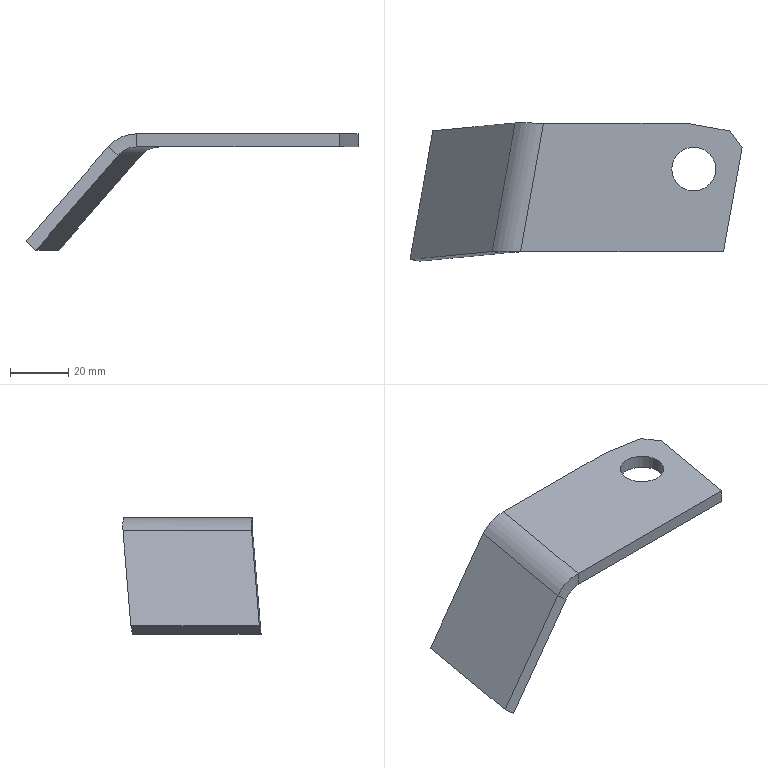Part | SolidWorks | features FlatPattern 1, SM3dBend 1, SMBaseFlange 1, SheetMetal 1 | 1 solid | 18 faces | box 113.633 x 47.299 x 39.859 mm | volume 23066 mm3 | plane 12 | cylinder 4 | spline 2 | commonest cylinder face diameters 15 x2 16 x1 25 x1
STEP:
#1=CARTESIAN_POINT('',(103.623,28.367,-4.5));
#2=VERTEX_POINT('',#1);
#3=CARTESIAN_POINT('',(118.623,28.367,-4.5));
#4=VERTEX_POINT('',#3);
#5=CARTESIAN_POINT('',(111.123,28.367,-4.5));
#6=DIRECTION('',(0.,0.,1.));
#7=DIRECTION('',(1.,0.,0.));
#8=AXIS2_PLACEMENT_3D('',#5,#6,#7);
#9=CIRCLE('',#8,7.5);
#10=EDGE_CURVE('',#2,#4,#9,.T.);
#11=ORIENTED_EDGE('',*,*,#10,.F.);
#12=CARTESIAN_POINT('',(103.623,28.367,0.));
#13=VERTEX_POINT('',#12);
#14=CARTESIAN_POINT('',(103.623,28.367,-4.5));
#15=DIRECTION('',(0.,0.,1.));
#16=VECTOR('',#15,1000.);
#17=LINE('',#14,#16);
#18=EDGE_CURVE('',#2,#13,#17,.T.);
#19=ORIENTED_EDGE('',*,*,#18,.T.);
#20=CARTESIAN_POINT('',(118.623,28.367,0.));
#21=VERTEX_POINT('',#20);
#22=CARTESIAN_POINT('',(111.123,28.367,0.));
#23=DIRECTION('',(0.,0.,1.));
#24=DIRECTION('',(1.,0.,0.));
#25=AXIS2_PLACEMENT_3D('',#22,#23,#24);
#26=CIRCLE('',#25,7.5);
#27=EDGE_CURVE('',#13,#21,#26,.T.);
#28=ORIENTED_EDGE('',*,*,#27,.T.);
#29=CARTESIAN_POINT('',(118.623,28.367,-4.5));
#30=DIRECTION('',(0.,0.,1.));
#31=VECTOR('',#30,1000.);
#32=LINE('',#29,#31);
#33=EDGE_CURVE('',#4,#21,#32,.T.);
#34=ORIENTED_EDGE('',*,*,#33,.F.);
#35=EDGE_LOOP('',(#11,#19,#28,#34));
#36=FACE_OUTER_BOUND('',#35,.T.);
#37=CARTESIAN_POINT('',(111.123,28.367,-4.5));
#38=DIRECTION('',(0.,0.,1.));
#39=DIRECTION('',(1.,0.,0.));
#40=AXIS2_PLACEMENT_3D('',#37,#38,#39);
#41=CYLINDRICAL_SURFACE('',#40,7.5);
#42=ADVANCED_FACE('',(#36),#41,.F.);
#43=CARTESIAN_POINT('',(53.399,43.554,-7.358));
#44=VERTEX_POINT('',#43);
#45=CARTESIAN_POINT('',(25.222,40.893,-39.859));
#46=VERTEX_POINT('',#45);
#47=CARTESIAN_POINT('',(91.322,47.135,36.385));
#48=DIRECTION('',(-0.6538,-0.06175,-0.7541));
#49=VECTOR('',#48,1000.);
#50=LINE('',#47,#49);
#51=EDGE_CURVE('',#44,#46,#50,.T.);
#52=ORIENTED_EDGE('',*,*,#51,.F.);
#53=CARTESIAN_POINT('',(45.551,-0.4463,-7.358));
#54=VERTEX_POINT('',#53);
#55=CARTESIAN_POINT('',(44.224,-7.888,-7.358));
#56=DIRECTION('',(-0.1756,-0.9845,0.));
#57=VECTOR('',#56,1000.);
#58=LINE('',#55,#57);
#59=EDGE_CURVE('',#44,#54,#58,.T.);
#60=ORIENTED_EDGE('',*,*,#59,.T.);
#61=CARTESIAN_POINT('',(17.406,-3.104,-39.823));
#62=VERTEX_POINT('',#61);
#63=CARTESIAN_POINT('',(17.406,-3.104,-39.823));
#64=DIRECTION('',(0.6538,0.06175,0.7541));
#65=VECTOR('',#64,1000.);
#66=LINE('',#63,#65);
#67=EDGE_CURVE('',#62,#54,#66,.T.);
#68=ORIENTED_EDGE('',*,*,#67,.F.);
#69=CARTESIAN_POINT('',(25.222,40.893,-39.859));
#70=DIRECTION('',(-0.1749,-0.9846,0.0008057));
#71=VECTOR('',#70,1000.);
#72=LINE('',#69,#71);
#73=EDGE_CURVE('',#46,#62,#72,.T.);
#74=ORIENTED_EDGE('',*,*,#73,.F.);
#75=EDGE_LOOP('',(#52,#60,#68,#74));
#76=FACE_OUTER_BOUND('',#75,.T.);
#77=CARTESIAN_POINT('',(17.406,-3.104,-39.823));
#78=DIRECTION('',(-0.7541,0.1345,0.6428));
#79=DIRECTION('',(0.6538,0.06175,0.7541));
#80=AXIS2_PLACEMENT_3D('',#77,#78,#79);
#81=PLANE('',#80);
#82=ADVANCED_FACE('',(#76),#81,.F.);
#83=CARTESIAN_POINT('',(21.829,41.498,-36.967));
#84=VERTEX_POINT('',#83);
#85=CARTESIAN_POINT('',(14.012,-2.499,-36.931));
#86=VERTEX_POINT('',#85);
#87=CARTESIAN_POINT('',(21.829,41.498,-36.967));
#88=DIRECTION('',(-0.1749,-0.9846,0.0008057));
#89=VECTOR('',#88,1000.);
#90=LINE('',#87,#89);
#91=EDGE_CURVE('',#84,#86,#90,.T.);
#92=ORIENTED_EDGE('',*,*,#91,.F.);
#93=CARTESIAN_POINT('',(25.222,40.893,-39.859));
#94=DIRECTION('',(-0.7541,0.1345,0.6428));
#95=VECTOR('',#94,1000.);
#96=LINE('',#93,#95);
#97=EDGE_CURVE('',#46,#84,#96,.T.);
#98=ORIENTED_EDGE('',*,*,#97,.F.);
#99=ORIENTED_EDGE('',*,*,#73,.T.);
#100=CARTESIAN_POINT('',(17.406,-3.104,-39.823));
#101=DIRECTION('',(-0.7541,0.1345,0.6428));
#102=VECTOR('',#101,1000.);
#103=LINE('',#100,#102);
#104=EDGE_CURVE('',#62,#86,#103,.T.);
#105=ORIENTED_EDGE('',*,*,#104,.T.);
#106=EDGE_LOOP('',(#92,#98,#99,#105));
#107=FACE_OUTER_BOUND('',#106,.T.);
#108=CARTESIAN_POINT('',(25.222,40.893,-39.859));
#109=DIRECTION('',(-0.633,0.1118,-0.766));
#110=DIRECTION('',(-0.1749,-0.9846,0.0008057));
#111=AXIS2_PLACEMENT_3D('',#108,#109,#110);
#112=PLANE('',#111);
#113=ADVANCED_FACE('',(#107),#112,.T.);
#114=CARTESIAN_POINT('',(50.006,44.159,-4.465));
#115=VERTEX_POINT('',#114);
#116=CARTESIAN_POINT('',(53.399,43.554,-7.358));
#117=CARTESIAN_POINT('',(50.006,44.159,-4.465));
#118=B_SPLINE_CURVE_WITH_KNOTS('',1,(#116,#117),.UNSPECIFIED.,.F.,.F.,(2,2),(0.,1.),.UNSPECIFIED.);
#119=EDGE_CURVE('',#44,#115,#118,.T.);
#120=ORIENTED_EDGE('',*,*,#119,.F.);
#121=ORIENTED_EDGE('',*,*,#51,.T.);
#122=ORIENTED_EDGE('',*,*,#97,.T.);
#123=CARTESIAN_POINT('',(87.928,47.741,39.277));
#124=DIRECTION('',(-0.6538,-0.06175,-0.7541));
#125=VECTOR('',#124,1000.);
#126=LINE('',#123,#125);
#127=EDGE_CURVE('',#115,#84,#126,.T.);
#128=ORIENTED_EDGE('',*,*,#127,.F.);
#129=EDGE_LOOP('',(#120,#121,#122,#128));
#130=FACE_OUTER_BOUND('',#129,.T.);
#131=CARTESIAN_POINT('',(91.322,47.135,36.385));
#132=DIRECTION('',(0.06175,0.989,-0.1345));
#133=DIRECTION('',(-0.6538,-0.06175,-0.7541));
#134=AXIS2_PLACEMENT_3D('',#131,#132,#133);
#135=PLANE('',#134);
#136=ADVANCED_FACE('',(#130),#135,.T.);
#137=CARTESIAN_POINT('',(42.158,0.159,-4.465));
#138=VERTEX_POINT('',#137);
#139=CARTESIAN_POINT('',(42.158,0.159,-4.465));
#140=CARTESIAN_POINT('',(45.551,-0.4463,-7.358));
#141=B_SPLINE_CURVE_WITH_KNOTS('',1,(#139,#140),.UNSPECIFIED.,.F.,.F.,(2,2),(0.,1.),.UNSPECIFIED.);
#142=EDGE_CURVE('',#138,#54,#141,.T.);
#143=ORIENTED_EDGE('',*,*,#142,.F.);
#144=CARTESIAN_POINT('',(14.012,-2.499,-36.931));
#145=DIRECTION('',(0.6538,0.06175,0.7541));
#146=VECTOR('',#145,1000.);
#147=LINE('',#144,#146);
#148=EDGE_CURVE('',#86,#138,#147,.T.);
#149=ORIENTED_EDGE('',*,*,#148,.F.);
#150=ORIENTED_EDGE('',*,*,#104,.F.);
#151=ORIENTED_EDGE('',*,*,#67,.T.);
#152=EDGE_LOOP('',(#143,#149,#150,#151));
#153=FACE_OUTER_BOUND('',#152,.T.);
#154=CARTESIAN_POINT('',(17.406,-3.104,-39.823));
#155=DIRECTION('',(-0.06175,-0.989,0.1345));
#156=DIRECTION('',(0.7541,-0.1345,-0.6428));
#157=AXIS2_PLACEMENT_3D('',#154,#155,#156);
#158=PLANE('',#157);
#159=ADVANCED_FACE('',(#153),#158,.T.);
#160=CARTESIAN_POINT('',(40.831,-7.282,-4.465));
#161=DIRECTION('',(-0.1756,-0.9845,0.));
#162=VECTOR('',#161,1000.);
#163=LINE('',#160,#162);
#164=EDGE_CURVE('',#115,#138,#163,.T.);
#165=ORIENTED_EDGE('',*,*,#164,.F.);
#166=ORIENTED_EDGE('',*,*,#127,.T.);
#167=ORIENTED_EDGE('',*,*,#91,.T.);
#168=ORIENTED_EDGE('',*,*,#148,.T.);
#169=EDGE_LOOP('',(#165,#166,#167,#168));
#170=FACE_OUTER_BOUND('',#169,.T.);
#171=CARTESIAN_POINT('',(14.012,-2.499,-36.931));
#172=DIRECTION('',(-0.7541,0.1345,0.6428));
#173=DIRECTION('',(0.6538,0.06175,0.7541));
#174=AXIS2_PLACEMENT_3D('',#171,#172,#173);
#175=PLANE('',#174);
#176=ADVANCED_FACE('',(#170),#175,.T.);
#177=ORIENTED_EDGE('',*,*,#18,.F.);
#178=CARTESIAN_POINT('',(111.123,28.367,-4.5));
#179=DIRECTION('',(0.,0.,1.));
#180=DIRECTION('',(1.,0.,0.));
#181=AXIS2_PLACEMENT_3D('',#178,#179,#180);
#182=CIRCLE('',#181,7.5);
#183=EDGE_CURVE('',#4,#2,#182,.T.);
#184=ORIENTED_EDGE('',*,*,#183,.F.);
#185=ORIENTED_EDGE('',*,*,#33,.T.);
#186=CARTESIAN_POINT('',(111.123,28.367,0.));
#187=DIRECTION('',(0.,0.,1.));
#188=DIRECTION('',(1.,0.,0.));
#189=AXIS2_PLACEMENT_3D('',#186,#187,#188);
#190=CIRCLE('',#189,7.5);
#191=EDGE_CURVE('',#21,#13,#190,.T.);
#192=ORIENTED_EDGE('',*,*,#191,.T.);
#193=EDGE_LOOP('',(#177,#184,#185,#192));
#194=FACE_OUTER_BOUND('',#193,.T.);
#195=CARTESIAN_POINT('',(111.123,28.367,-4.5));
#196=DIRECTION('',(0.,0.,1.));
#197=DIRECTION('',(1.,0.,0.));
#198=AXIS2_PLACEMENT_3D('',#195,#196,#197);
#199=CYLINDRICAL_SURFACE('',#198,7.5);
#200=ADVANCED_FACE('',(#194),#199,.F.);
#201=CARTESIAN_POINT('',(121.3,0.,0.));
#202=VERTEX_POINT('',#201);
#203=CARTESIAN_POINT('',(127.646,35.578,0.));
#204=VERTEX_POINT('',#203);
#205=CARTESIAN_POINT('',(121.3,0.,0.));
#206=DIRECTION('',(0.1756,0.9845,0.));
#207=VECTOR('',#206,1000.);
#208=LINE('',#205,#207);
#209=EDGE_CURVE('',#202,#204,#208,.T.);
#210=ORIENTED_EDGE('',*,*,#209,.F.);
#211=CARTESIAN_POINT('',(121.3,0.,-4.5));
#212=VERTEX_POINT('',#211);
#213=CARTESIAN_POINT('',(121.3,0.,-4.5));
#214=DIRECTION('',(0.,0.,1.));
#215=VECTOR('',#214,1000.);
#216=LINE('',#213,#215);
#217=EDGE_CURVE('',#212,#202,#216,.T.);
#218=ORIENTED_EDGE('',*,*,#217,.F.);
#219=CARTESIAN_POINT('',(127.646,35.578,-4.5));
#220=VERTEX_POINT('',#219);
#221=CARTESIAN_POINT('',(121.3,0.,-4.5));
#222=DIRECTION('',(0.1756,0.9845,0.));
#223=VECTOR('',#222,1000.);
#224=LINE('',#221,#223);
#225=EDGE_CURVE('',#212,#220,#224,.T.);
#226=ORIENTED_EDGE('',*,*,#225,.T.);
#227=CARTESIAN_POINT('',(127.646,35.578,-4.5));
#228=DIRECTION('',(0.,0.,1.));
#229=VECTOR('',#228,1000.);
#230=LINE('',#227,#229);
#231=EDGE_CURVE('',#220,#204,#230,.T.);
#232=ORIENTED_EDGE('',*,*,#231,.T.);
#233=EDGE_LOOP('',(#210,#218,#226,#232));
#234=FACE_OUTER_BOUND('',#233,.T.);
#235=CARTESIAN_POINT('',(121.3,0.,-4.5));
#236=DIRECTION('',(0.9845,-0.1756,0.));
#237=DIRECTION('',(0.1756,0.9845,0.));
#238=AXIS2_PLACEMENT_3D('',#235,#236,#237);
#239=PLANE('',#238);
#240=ADVANCED_FACE('',(#234),#239,.T.);
#241=CARTESIAN_POINT('',(123.601,41.378,0.));
#242=VERTEX_POINT('',#241);
#243=CARTESIAN_POINT('',(123.601,41.378,0.));
#244=DIRECTION('',(-0.572,0.8203,0.));
#245=VECTOR('',#244,1000.);
#246=LINE('',#243,#245);
#247=EDGE_CURVE('',#204,#242,#246,.T.);
#248=ORIENTED_EDGE('',*,*,#247,.F.);
#249=ORIENTED_EDGE('',*,*,#231,.F.);
#250=CARTESIAN_POINT('',(123.601,41.378,-4.5));
#251=VERTEX_POINT('',#250);
#252=CARTESIAN_POINT('',(123.601,41.378,-4.5));
#253=DIRECTION('',(-0.572,0.8203,0.));
#254=VECTOR('',#253,1000.);
#255=LINE('',#252,#254);
#256=EDGE_CURVE('',#220,#251,#255,.T.);
#257=ORIENTED_EDGE('',*,*,#256,.T.);
#258=CARTESIAN_POINT('',(123.601,41.378,-4.5));
#259=DIRECTION('',(0.,0.,1.));
#260=VECTOR('',#259,1000.);
#261=LINE('',#258,#260);
#262=EDGE_CURVE('',#251,#242,#261,.T.);
#263=ORIENTED_EDGE('',*,*,#262,.T.);
#264=EDGE_LOOP('',(#248,#249,#257,#263));
#265=FACE_OUTER_BOUND('',#264,.T.);
#266=CARTESIAN_POINT('',(123.601,41.378,-4.5));
#267=DIRECTION('',(0.8203,0.572,0.));
#268=DIRECTION('',(-0.572,0.8203,0.));
#269=AXIS2_PLACEMENT_3D('',#266,#267,#268);
#270=PLANE('',#269);
#271=ADVANCED_FACE('',(#265),#270,.T.);
#272=CARTESIAN_POINT('',(108.9,44.,0.));
#273=VERTEX_POINT('',#272);
#274=CARTESIAN_POINT('',(108.9,44.,0.));
#275=DIRECTION('',(-0.9845,0.1756,0.));
#276=VECTOR('',#275,1000.);
#277=LINE('',#274,#276);
#278=EDGE_CURVE('',#242,#273,#277,.T.);
#279=ORIENTED_EDGE('',*,*,#278,.F.);
#280=ORIENTED_EDGE('',*,*,#262,.F.);
#281=CARTESIAN_POINT('',(108.9,44.,-4.5));
#282=VERTEX_POINT('',#281);
#283=CARTESIAN_POINT('',(108.9,44.,-4.5));
#284=DIRECTION('',(-0.9845,0.1756,0.));
#285=VECTOR('',#284,1000.);
#286=LINE('',#283,#285);
#287=EDGE_CURVE('',#251,#282,#286,.T.);
#288=ORIENTED_EDGE('',*,*,#287,.T.);
#289=CARTESIAN_POINT('',(108.9,44.,-4.5));
#290=DIRECTION('',(0.,0.,1.));
#291=VECTOR('',#290,1000.);
#292=LINE('',#289,#291);
#293=EDGE_CURVE('',#282,#273,#292,.T.);
#294=ORIENTED_EDGE('',*,*,#293,.T.);
#295=EDGE_LOOP('',(#279,#280,#288,#294));
#296=FACE_OUTER_BOUND('',#295,.T.);
#297=CARTESIAN_POINT('',(108.9,44.,-4.5));
#298=DIRECTION('',(0.1756,0.9845,0.));
#299=DIRECTION('',(-0.9845,0.1756,0.));
#300=AXIS2_PLACEMENT_3D('',#297,#298,#299);
#301=PLANE('',#300);
#302=ADVANCED_FACE('',(#296),#301,.T.);
#303=CARTESIAN_POINT('',(59.704,44.,-4.5));
#304=VERTEX_POINT('',#303);
#305=CARTESIAN_POINT('',(51.856,0.,-4.5));
#306=VERTEX_POINT('',#305);
#307=CARTESIAN_POINT('',(50.257,-8.964,-4.5));
#308=DIRECTION('',(-0.1756,-0.9845,0.));
#309=VECTOR('',#308,1000.);
#310=LINE('',#307,#309);
#311=EDGE_CURVE('',#304,#306,#310,.T.);
#312=ORIENTED_EDGE('',*,*,#311,.F.);
#313=CARTESIAN_POINT('',(108.9,44.,-4.5));
#314=DIRECTION('',(-1.,0.,0.));
#315=VECTOR('',#314,1000.);
#316=LINE('',#313,#315);
#317=EDGE_CURVE('',#282,#304,#316,.T.);
#318=ORIENTED_EDGE('',*,*,#317,.F.);
#319=ORIENTED_EDGE('',*,*,#287,.F.);
#320=ORIENTED_EDGE('',*,*,#256,.F.);
#321=ORIENTED_EDGE('',*,*,#225,.F.);
#322=CARTESIAN_POINT('',(0.,0.,-4.5));
#323=DIRECTION('',(1.,0.,0.));
#324=VECTOR('',#323,1000.);
#325=LINE('',#322,#324);
#326=EDGE_CURVE('',#306,#212,#325,.T.);
#327=ORIENTED_EDGE('',*,*,#326,.F.);
#328=EDGE_LOOP('',(#312,#318,#319,#320,#321,#327));
#329=FACE_OUTER_BOUND('',#328,.T.);
#330=ORIENTED_EDGE('',*,*,#183,.T.);
#331=ORIENTED_EDGE('',*,*,#10,.T.);
#332=EDGE_LOOP('',(#330,#331));
#333=FACE_BOUND('',#332,.T.);
#334=CARTESIAN_POINT('',(0.,0.,-4.5));
#335=DIRECTION('',(0.,0.,1.));
#336=DIRECTION('',(1.,0.,0.));
#337=AXIS2_PLACEMENT_3D('',#334,#335,#336);
#338=PLANE('',#337);
#339=ADVANCED_FACE('',(#329,#333),#338,.F.);
#340=ORIENTED_EDGE('',*,*,#317,.T.);
#341=CARTESIAN_POINT('',(59.704,44.,0.));
#342=VERTEX_POINT('',#341);
#343=CARTESIAN_POINT('',(59.704,44.,-4.5));
#344=CARTESIAN_POINT('',(59.704,44.,-3.));
#345=CARTESIAN_POINT('',(59.704,44.,-1.5));
#346=CARTESIAN_POINT('',(59.704,44.,0.));
#347=B_SPLINE_CURVE_WITH_KNOTS('',3,(#343,#344,#345,#346),.UNSPECIFIED.,.F.,.F.,(4,4),(0.,1.),.UNSPECIFIED.);
#348=EDGE_CURVE('',#304,#342,#347,.T.);
#349=ORIENTED_EDGE('',*,*,#348,.T.);
#350=CARTESIAN_POINT('',(108.9,44.,0.));
#351=DIRECTION('',(-1.,0.,0.));
#352=VECTOR('',#351,1000.);
#353=LINE('',#350,#352);
#354=EDGE_CURVE('',#273,#342,#353,.T.);
#355=ORIENTED_EDGE('',*,*,#354,.F.);
#356=ORIENTED_EDGE('',*,*,#293,.F.);
#357=EDGE_LOOP('',(#340,#349,#355,#356));
#358=FACE_OUTER_BOUND('',#357,.T.);
#359=CARTESIAN_POINT('',(108.9,44.,-4.5));
#360=DIRECTION('',(0.,1.,0.));
#361=DIRECTION('',(-1.,0.,0.));
#362=AXIS2_PLACEMENT_3D('',#359,#360,#361);
#363=PLANE('',#362);
#364=ADVANCED_FACE('',(#358),#363,.T.);
#365=ORIENTED_EDGE('',*,*,#191,.F.);
#366=ORIENTED_EDGE('',*,*,#27,.F.);
#367=EDGE_LOOP('',(#365,#366));
#368=FACE_BOUND('',#367,.T.);
#369=ORIENTED_EDGE('',*,*,#354,.T.);
#370=CARTESIAN_POINT('',(51.856,0.,0.));
#371=VERTEX_POINT('',#370);
#372=CARTESIAN_POINT('',(50.257,-8.964,0.));
#373=DIRECTION('',(-0.1756,-0.9845,0.));
#374=VECTOR('',#373,1000.);
#375=LINE('',#372,#374);
#376=EDGE_CURVE('',#342,#371,#375,.T.);
#377=ORIENTED_EDGE('',*,*,#376,.T.);
#378=CARTESIAN_POINT('',(0.,0.,0.));
#379=DIRECTION('',(1.,0.,0.));
#380=VECTOR('',#379,1000.);
#381=LINE('',#378,#380);
#382=EDGE_CURVE('',#371,#202,#381,.T.);
#383=ORIENTED_EDGE('',*,*,#382,.T.);
#384=ORIENTED_EDGE('',*,*,#209,.T.);
#385=ORIENTED_EDGE('',*,*,#247,.T.);
#386=ORIENTED_EDGE('',*,*,#278,.T.);
#387=EDGE_LOOP('',(#369,#377,#383,#384,#385,#386));
#388=FACE_OUTER_BOUND('',#387,.T.);
#389=CARTESIAN_POINT('',(0.,0.,0.));
#390=DIRECTION('',(0.,0.,1.));
#391=DIRECTION('',(1.,0.,0.));
#392=AXIS2_PLACEMENT_3D('',#389,#390,#391);
#393=PLANE('',#392);
#394=ADVANCED_FACE('',(#368,#388),#393,.T.);
#395=ORIENTED_EDGE('',*,*,#382,.F.);
#396=CARTESIAN_POINT('',(51.856,0.,0.));
#397=CARTESIAN_POINT('',(51.856,0.,-1.5));
#398=CARTESIAN_POINT('',(51.856,0.,-3.));
#399=CARTESIAN_POINT('',(51.856,0.,-4.5));
#400=B_SPLINE_CURVE_WITH_KNOTS('',3,(#396,#397,#398,#399),.UNSPECIFIED.,.F.,.F.,(4,4),(0.,1.),.UNSPECIFIED.);
#401=EDGE_CURVE('',#371,#306,#400,.T.);
#402=ORIENTED_EDGE('',*,*,#401,.T.);
#403=ORIENTED_EDGE('',*,*,#326,.T.);
#404=ORIENTED_EDGE('',*,*,#217,.T.);
#405=EDGE_LOOP('',(#395,#402,#403,#404));
#406=FACE_OUTER_BOUND('',#405,.T.);
#407=CARTESIAN_POINT('',(0.,0.,-4.5));
#408=DIRECTION('',(0.,-1.,0.));
#409=DIRECTION('',(0.,0.,-1.));
#410=AXIS2_PLACEMENT_3D('',#407,#408,#409);
#411=PLANE('',#410);
#412=ADVANCED_FACE('',(#406),#411,.T.);
#413=ORIENTED_EDGE('',*,*,#119,.T.);
#414=CARTESIAN_POINT('',(50.006,44.159,-4.465));
#415=CARTESIAN_POINT('',(51.202,44.208,-3.072));
#416=CARTESIAN_POINT('',(52.7,44.202,-1.939));
#417=CARTESIAN_POINT('',(56.035,44.131,-0.4028));
#418=CARTESIAN_POINT('',(57.868,44.066,0.));
#419=CARTESIAN_POINT('',(59.704,44.,0.));
#420=B_SPLINE_CURVE_WITH_KNOTS('',3,(#414,#415,#416,#417,#418,#419),.UNSPECIFIED.,.F.,.F.,(4,2,4),(0.,0.5,1.),.UNSPECIFIED.);
#421=EDGE_CURVE('',#115,#342,#420,.T.);
#422=ORIENTED_EDGE('',*,*,#421,.T.);
#423=ORIENTED_EDGE('',*,*,#348,.F.);
#424=CARTESIAN_POINT('',(53.399,43.554,-7.358));
#425=CARTESIAN_POINT('',(54.181,43.676,-6.466));
#426=CARTESIAN_POINT('',(55.156,43.764,-5.741));
#427=CARTESIAN_POINT('',(57.323,43.901,-4.758));
#428=CARTESIAN_POINT('',(58.513,43.951,-4.5));
#429=CARTESIAN_POINT('',(59.704,44.,-4.5));
#430=B_SPLINE_CURVE_WITH_KNOTS('',3,(#424,#425,#426,#427,#428,#429),.UNSPECIFIED.,.F.,.F.,(4,2,4),(0.,0.5,1.),.UNSPECIFIED.);
#431=EDGE_CURVE('',#44,#304,#430,.T.);
#432=ORIENTED_EDGE('',*,*,#431,.F.);
#433=EDGE_LOOP('',(#413,#422,#423,#432));
#434=FACE_OUTER_BOUND('',#433,.T.);
#435=CARTESIAN_POINT('',(50.006,44.159,-4.465));
#436=CARTESIAN_POINT('',(51.202,44.208,-3.072));
#437=CARTESIAN_POINT('',(52.7,44.202,-1.939));
#438=CARTESIAN_POINT('',(56.035,44.131,-0.4028));
#439=CARTESIAN_POINT('',(57.868,44.066,0.));
#440=CARTESIAN_POINT('',(59.704,44.,0.));
#441=CARTESIAN_POINT('',(53.399,43.554,-7.358));
#442=CARTESIAN_POINT('',(54.181,43.676,-6.466));
#443=CARTESIAN_POINT('',(55.156,43.764,-5.741));
#444=CARTESIAN_POINT('',(57.323,43.901,-4.758));
#445=CARTESIAN_POINT('',(58.513,43.951,-4.5));
#446=CARTESIAN_POINT('',(59.704,44.,-4.5));
#447=B_SPLINE_SURFACE_WITH_KNOTS('',1,3,((#435,#436,#437,#438,#439,#440),(#441,#442,#443,#444,#445,#446)),.UNSPECIFIED.,.F.,.F.,.F.,(2,2),(4,2,4),(0.,1.),(0.,0.5,1.),.UNSPECIFIED.);
#448=ADVANCED_FACE('',(#434),#447,.F.);
#449=ORIENTED_EDGE('',*,*,#401,.F.);
#450=CARTESIAN_POINT('',(51.856,0.,0.));
#451=CARTESIAN_POINT('',(50.021,0.06552,0.));
#452=CARTESIAN_POINT('',(48.187,0.1308,-0.4028));
#453=CARTESIAN_POINT('',(44.852,0.202,-1.939));
#454=CARTESIAN_POINT('',(43.354,0.2076,-3.072));
#455=CARTESIAN_POINT('',(42.158,0.159,-4.465));
#456=B_SPLINE_CURVE_WITH_KNOTS('',3,(#450,#451,#452,#453,#454,#455),.UNSPECIFIED.,.F.,.F.,(4,2,4),(0.,0.5,1.),.UNSPECIFIED.);
#457=EDGE_CURVE('',#371,#138,#456,.T.);
#458=ORIENTED_EDGE('',*,*,#457,.T.);
#459=ORIENTED_EDGE('',*,*,#142,.T.);
#460=CARTESIAN_POINT('',(51.856,0.,-4.5));
#461=CARTESIAN_POINT('',(50.665,-0.04942,-4.5));
#462=CARTESIAN_POINT('',(49.475,-0.09895,-4.758));
#463=CARTESIAN_POINT('',(47.308,-0.2361,-5.741));
#464=CARTESIAN_POINT('',(46.333,-0.3239,-6.466));
#465=CARTESIAN_POINT('',(45.551,-0.4463,-7.358));
#466=B_SPLINE_CURVE_WITH_KNOTS('',3,(#460,#461,#462,#463,#464,#465),.UNSPECIFIED.,.F.,.F.,(4,2,4),(0.,0.5,1.),.UNSPECIFIED.);
#467=EDGE_CURVE('',#306,#54,#466,.T.);
#468=ORIENTED_EDGE('',*,*,#467,.F.);
#469=EDGE_LOOP('',(#449,#458,#459,#468));
#470=FACE_OUTER_BOUND('',#469,.T.);
#471=CARTESIAN_POINT('',(51.856,0.,0.));
#472=CARTESIAN_POINT('',(50.021,0.06552,0.));
#473=CARTESIAN_POINT('',(48.187,0.1308,-0.4028));
#474=CARTESIAN_POINT('',(44.852,0.202,-1.939));
#475=CARTESIAN_POINT('',(43.354,0.2076,-3.072));
#476=CARTESIAN_POINT('',(42.158,0.159,-4.465));
#477=CARTESIAN_POINT('',(51.856,0.,-4.5));
#478=CARTESIAN_POINT('',(50.665,-0.04943,-4.5));
#479=CARTESIAN_POINT('',(49.475,-0.09895,-4.758));
#480=CARTESIAN_POINT('',(47.308,-0.2361,-5.741));
#481=CARTESIAN_POINT('',(46.333,-0.3238,-6.466));
#482=CARTESIAN_POINT('',(45.551,-0.4463,-7.358));
#483=B_SPLINE_SURFACE_WITH_KNOTS('',1,3,((#471,#472,#473,#474,#475,#476),(#477,#478,#479,#480,#481,#482)),.UNSPECIFIED.,.F.,.F.,.F.,(2,2),(4,2,4),(0.,1.),(0.,0.5,1.),.UNSPECIFIED.);
#484=ADVANCED_FACE('',(#470),#483,.F.);
#485=ORIENTED_EDGE('',*,*,#467,.T.);
#486=ORIENTED_EDGE('',*,*,#59,.F.);
#487=ORIENTED_EDGE('',*,*,#431,.T.);
#488=ORIENTED_EDGE('',*,*,#311,.T.);
#489=EDGE_LOOP('',(#485,#486,#487,#488));
#490=FACE_OUTER_BOUND('',#489,.T.);
#491=CARTESIAN_POINT('',(47.482,-24.527,-12.5));
#492=DIRECTION('',(0.1756,0.9845,0.));
#493=DIRECTION('',(-0.9845,0.1756,0.));
#494=AXIS2_PLACEMENT_3D('',#491,#492,#493);
#495=CYLINDRICAL_SURFACE('',#494,8.);
#496=ADVANCED_FACE('',(#490),#495,.F.);
#497=ORIENTED_EDGE('',*,*,#457,.F.);
#498=ORIENTED_EDGE('',*,*,#376,.F.);
#499=ORIENTED_EDGE('',*,*,#421,.F.);
#500=ORIENTED_EDGE('',*,*,#164,.T.);
#501=EDGE_LOOP('',(#497,#498,#499,#500));
#502=FACE_OUTER_BOUND('',#501,.T.);
#503=CARTESIAN_POINT('',(47.482,-24.527,-12.5));
#504=DIRECTION('',(0.1756,0.9845,0.));
#505=DIRECTION('',(-0.9845,0.1756,0.));
#506=AXIS2_PLACEMENT_3D('',#503,#504,#505);
#507=CYLINDRICAL_SURFACE('',#506,12.5);
#508=ADVANCED_FACE('',(#502),#507,.T.);
#509=CLOSED_SHELL('',(#42,#82,#113,#136,#159,#176,#200,#240,#271,#302,#339,#364,#394,#412,#448,#484,#496,#508));
#510=MANIFOLD_SOLID_BREP('',#509);
#511=CARTESIAN_POINT('',(0.,0.,0.));
#512=DIRECTION('',(0.,0.,1.));
#513=DIRECTION('',(1.,0.,0.));
#514=AXIS2_PLACEMENT_3D('',#511,#512,#513);
#515=(LENGTH_UNIT()NAMED_UNIT(*)SI_UNIT(.MILLI.,.METRE.));
#516=UNCERTAINTY_MEASURE_WITH_UNIT(LENGTH_MEASURE(0.00001),#515,'','');
#517=(NAMED_UNIT(*)PLANE_ANGLE_UNIT()SI_UNIT($,.RADIAN.));
#518=(NAMED_UNIT(*)SI_UNIT($,.STERADIAN.)SOLID_ANGLE_UNIT());
#519=(GEOMETRIC_REPRESENTATION_CONTEXT(3)GLOBAL_UNCERTAINTY_ASSIGNED_CONTEXT((#516))GLOBAL_UNIT_ASSIGNED_CONTEXT((#515,#517,#518))REPRESENTATION_CONTEXT('',''));
#520=ADVANCED_BREP_SHAPE_REPRESENTATION('',(#510,#514),#519);